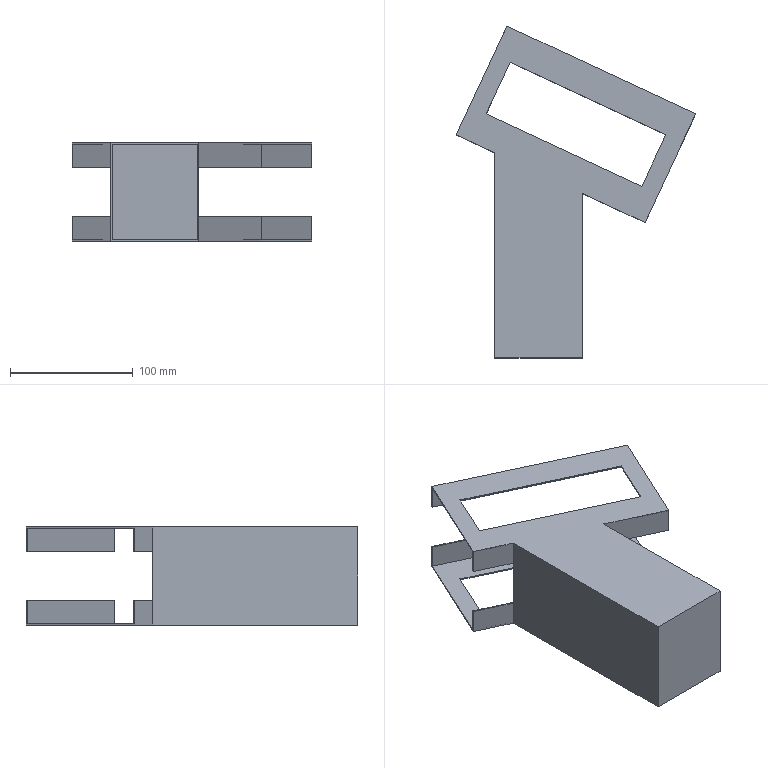Part | STEP file | Part3_4 | 1 solid | 44 faces | box 195.46 x 270.819 x 80 mm | volume 83841 mm3 | plane 44